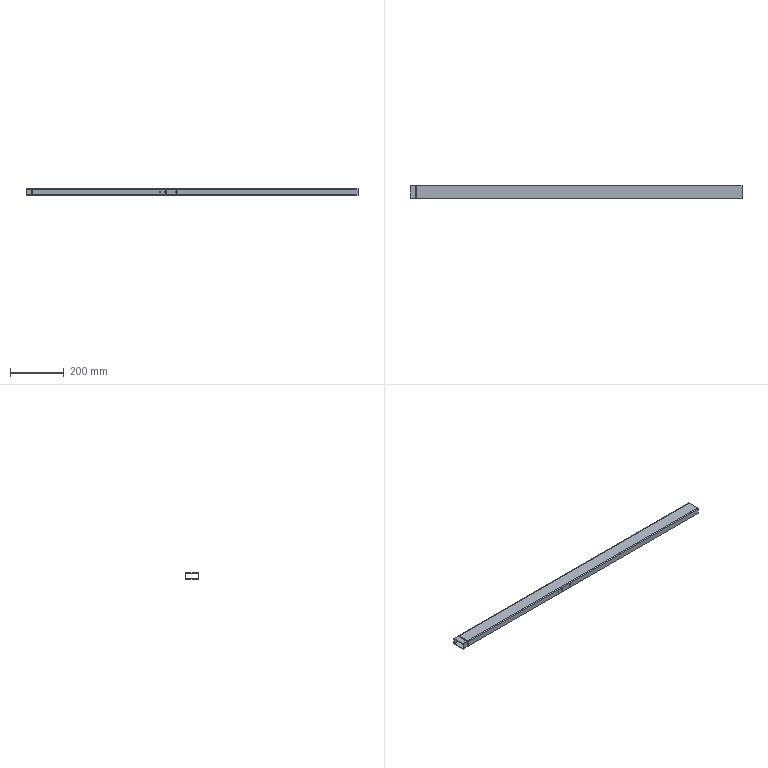Part | STEP file | 6100510 | 2 solids | 42 faces | box 1235 x 50 x 25 mm | volume 261105 mm3 | cylinder 22 | plane 20 | commonest cylinder face diameters 3 x8 5 x8 8 x4 3.2 x2